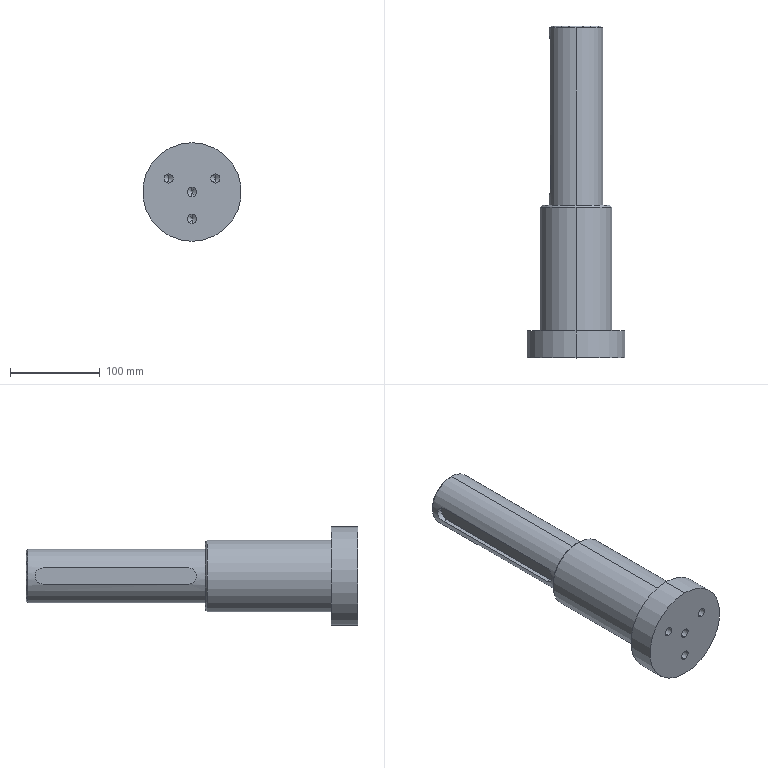Part | SolidWorks | features HoleWzd 2, ICE 2, Chamfer 1, Fillet 1, Revolution 1 | 1 solid | 41 faces | box 110 x 370 x 110 mm | volume 1516861 mm3 | cylinder 20 | cone 14 | plane 7 | commonest cylinder face diameters 10.2 x8 18 x4 15.5 x2 60 x2 80 x2 110 x2
STEP:
#1=CARTESIAN_POINT('',(0.,32.75,-24.9));
#2=VERTEX_POINT('',#1);
#3=CARTESIAN_POINT('',(0.,32.75,-35.1));
#4=VERTEX_POINT('',#3);
#5=CARTESIAN_POINT('',(0.,32.75,-30.));
#6=DIRECTION('',(0.,-1.,0.));
#7=DIRECTION('',(0.,0.,-1.));
#8=AXIS2_PLACEMENT_3D('',#5,#6,#7);
#9=CIRCLE('',#8,5.1);
#10=EDGE_CURVE('',#2,#4,#9,.T.);
#11=ORIENTED_EDGE('',*,*,#10,.F.);
#12=CARTESIAN_POINT('',(0.,0.,-24.9));
#13=VERTEX_POINT('',#12);
#14=CARTESIAN_POINT('',(0.,0.,-24.9));
#15=DIRECTION('',(0.,-1.,0.));
#16=VECTOR('',#15,1000.);
#17=LINE('',#14,#16);
#18=EDGE_CURVE('',#2,#13,#17,.T.);
#19=ORIENTED_EDGE('',*,*,#18,.T.);
#20=CARTESIAN_POINT('',(0.,0.,-35.1));
#21=VERTEX_POINT('',#20);
#22=CARTESIAN_POINT('',(0.,0.,-30.));
#23=DIRECTION('',(0.,-1.,0.));
#24=DIRECTION('',(0.,0.,-1.));
#25=AXIS2_PLACEMENT_3D('',#22,#23,#24);
#26=CIRCLE('',#25,5.1);
#27=EDGE_CURVE('',#13,#21,#26,.T.);
#28=ORIENTED_EDGE('',*,*,#27,.T.);
#29=CARTESIAN_POINT('',(0.,0.,-35.1));
#30=DIRECTION('',(0.,-1.,0.));
#31=VECTOR('',#30,1000.);
#32=LINE('',#29,#31);
#33=EDGE_CURVE('',#4,#21,#32,.T.);
#34=ORIENTED_EDGE('',*,*,#33,.F.);
#35=EDGE_LOOP('',(#11,#19,#28,#34));
#36=FACE_OUTER_BOUND('',#35,.T.);
#37=CARTESIAN_POINT('',(0.,0.,-30.));
#38=DIRECTION('',(0.,-1.,0.));
#39=DIRECTION('',(0.,0.,-1.));
#40=AXIS2_PLACEMENT_3D('',#37,#38,#39);
#41=CYLINDRICAL_SURFACE('',#40,5.1);
#42=ADVANCED_FACE('',(#36),#41,.F.);
#43=CARTESIAN_POINT('',(-25.981,32.75,20.1));
#44=VERTEX_POINT('',#43);
#45=CARTESIAN_POINT('',(-25.981,32.75,9.9));
#46=VERTEX_POINT('',#45);
#47=CARTESIAN_POINT('',(-25.981,32.75,15.));
#48=DIRECTION('',(0.,-1.,0.));
#49=DIRECTION('',(0.,0.,-1.));
#50=AXIS2_PLACEMENT_3D('',#47,#48,#49);
#51=CIRCLE('',#50,5.1);
#52=EDGE_CURVE('',#44,#46,#51,.T.);
#53=ORIENTED_EDGE('',*,*,#52,.F.);
#54=CARTESIAN_POINT('',(-25.981,0.,20.1));
#55=VERTEX_POINT('',#54);
#56=CARTESIAN_POINT('',(-25.981,0.,20.1));
#57=DIRECTION('',(0.,-1.,0.));
#58=VECTOR('',#57,1000.);
#59=LINE('',#56,#58);
#60=EDGE_CURVE('',#44,#55,#59,.T.);
#61=ORIENTED_EDGE('',*,*,#60,.T.);
#62=CARTESIAN_POINT('',(-25.981,0.,9.9));
#63=VERTEX_POINT('',#62);
#64=CARTESIAN_POINT('',(-25.981,0.,15.));
#65=DIRECTION('',(0.,-1.,0.));
#66=DIRECTION('',(0.,0.,-1.));
#67=AXIS2_PLACEMENT_3D('',#64,#65,#66);
#68=CIRCLE('',#67,5.1);
#69=EDGE_CURVE('',#55,#63,#68,.T.);
#70=ORIENTED_EDGE('',*,*,#69,.T.);
#71=CARTESIAN_POINT('',(-25.981,0.,9.9));
#72=DIRECTION('',(0.,-1.,0.));
#73=VECTOR('',#72,1000.);
#74=LINE('',#71,#73);
#75=EDGE_CURVE('',#46,#63,#74,.T.);
#76=ORIENTED_EDGE('',*,*,#75,.F.);
#77=EDGE_LOOP('',(#53,#61,#70,#76));
#78=FACE_OUTER_BOUND('',#77,.T.);
#79=CARTESIAN_POINT('',(-25.981,0.,15.));
#80=DIRECTION('',(0.,-1.,0.));
#81=DIRECTION('',(0.,0.,-1.));
#82=AXIS2_PLACEMENT_3D('',#79,#80,#81);
#83=CYLINDRICAL_SURFACE('',#82,5.1);
#84=ADVANCED_FACE('',(#78),#83,.F.);
#85=CARTESIAN_POINT('',(25.981,32.75,20.1));
#86=VERTEX_POINT('',#85);
#87=CARTESIAN_POINT('',(25.981,32.75,9.9));
#88=VERTEX_POINT('',#87);
#89=CARTESIAN_POINT('',(25.981,32.75,15.));
#90=DIRECTION('',(0.,-1.,0.));
#91=DIRECTION('',(0.,0.,-1.));
#92=AXIS2_PLACEMENT_3D('',#89,#90,#91);
#93=CIRCLE('',#92,5.1);
#94=EDGE_CURVE('',#86,#88,#93,.T.);
#95=ORIENTED_EDGE('',*,*,#94,.F.);
#96=CARTESIAN_POINT('',(25.981,0.,20.1));
#97=VERTEX_POINT('',#96);
#98=CARTESIAN_POINT('',(25.981,0.,20.1));
#99=DIRECTION('',(0.,-1.,0.));
#100=VECTOR('',#99,1000.);
#101=LINE('',#98,#100);
#102=EDGE_CURVE('',#86,#97,#101,.T.);
#103=ORIENTED_EDGE('',*,*,#102,.T.);
#104=CARTESIAN_POINT('',(25.981,0.,9.9));
#105=VERTEX_POINT('',#104);
#106=CARTESIAN_POINT('',(25.981,0.,15.));
#107=DIRECTION('',(0.,-1.,0.));
#108=DIRECTION('',(0.,0.,-1.));
#109=AXIS2_PLACEMENT_3D('',#106,#107,#108);
#110=CIRCLE('',#109,5.1);
#111=EDGE_CURVE('',#97,#105,#110,.T.);
#112=ORIENTED_EDGE('',*,*,#111,.T.);
#113=CARTESIAN_POINT('',(25.981,0.,9.9));
#114=DIRECTION('',(0.,-1.,0.));
#115=VECTOR('',#114,1000.);
#116=LINE('',#113,#115);
#117=EDGE_CURVE('',#88,#105,#116,.T.);
#118=ORIENTED_EDGE('',*,*,#117,.F.);
#119=EDGE_LOOP('',(#95,#103,#112,#118));
#120=FACE_OUTER_BOUND('',#119,.T.);
#121=CARTESIAN_POINT('',(25.981,0.,15.));
#122=DIRECTION('',(0.,-1.,0.));
#123=DIRECTION('',(0.,0.,-1.));
#124=AXIS2_PLACEMENT_3D('',#121,#122,#123);
#125=CYLINDRICAL_SURFACE('',#124,5.1);
#126=ADVANCED_FACE('',(#120),#125,.F.);
#127=CARTESIAN_POINT('',(0.,32.75,5.1));
#128=VERTEX_POINT('',#127);
#129=CARTESIAN_POINT('',(0.,32.75,-5.1));
#130=VERTEX_POINT('',#129);
#131=CARTESIAN_POINT('',(0.,32.75,0.));
#132=DIRECTION('',(0.,-1.,0.));
#133=DIRECTION('',(0.,0.,-1.));
#134=AXIS2_PLACEMENT_3D('',#131,#132,#133);
#135=CIRCLE('',#134,5.1);
#136=EDGE_CURVE('',#128,#130,#135,.T.);
#137=ORIENTED_EDGE('',*,*,#136,.F.);
#138=CARTESIAN_POINT('',(0.,0.,5.1));
#139=VERTEX_POINT('',#138);
#140=CARTESIAN_POINT('',(0.,0.,5.1));
#141=DIRECTION('',(0.,-1.,0.));
#142=VECTOR('',#141,1000.);
#143=LINE('',#140,#142);
#144=EDGE_CURVE('',#128,#139,#143,.T.);
#145=ORIENTED_EDGE('',*,*,#144,.T.);
#146=CARTESIAN_POINT('',(0.,0.,-5.1));
#147=VERTEX_POINT('',#146);
#148=CARTESIAN_POINT('',(0.,0.,0.));
#149=DIRECTION('',(0.,-1.,0.));
#150=DIRECTION('',(0.,0.,-1.));
#151=AXIS2_PLACEMENT_3D('',#148,#149,#150);
#152=CIRCLE('',#151,5.1);
#153=EDGE_CURVE('',#139,#147,#152,.T.);
#154=ORIENTED_EDGE('',*,*,#153,.T.);
#155=CARTESIAN_POINT('',(0.,0.,-5.1));
#156=DIRECTION('',(0.,-1.,0.));
#157=VECTOR('',#156,1000.);
#158=LINE('',#155,#157);
#159=EDGE_CURVE('',#130,#147,#158,.T.);
#160=ORIENTED_EDGE('',*,*,#159,.F.);
#161=EDGE_LOOP('',(#137,#145,#154,#160));
#162=FACE_OUTER_BOUND('',#161,.T.);
#163=CARTESIAN_POINT('',(0.,0.,0.));
#164=DIRECTION('',(0.,-1.,0.));
#165=DIRECTION('',(0.,0.,-1.));
#166=AXIS2_PLACEMENT_3D('',#163,#164,#165);
#167=CYLINDRICAL_SURFACE('',#166,5.1);
#168=ADVANCED_FACE('',(#162),#167,.F.);
#169=CARTESIAN_POINT('',(0.,35.814,-30.));
#170=VERTEX_POINT('',#169);
#171=CARTESIAN_POINT('',(0.,32.75,-35.1));
#172=DIRECTION('',(0.,-0.515,-0.8572));
#173=VECTOR('',#172,1000.);
#174=LINE('',#171,#173);
#175=EDGE_CURVE('',#170,#4,#174,.T.);
#176=ORIENTED_EDGE('',*,*,#175,.F.);
#177=CARTESIAN_POINT('',(0.,32.75,-24.9));
#178=DIRECTION('',(0.,-0.515,0.8572));
#179=VECTOR('',#178,1000.);
#180=LINE('',#177,#179);
#181=EDGE_CURVE('',#170,#2,#180,.T.);
#182=ORIENTED_EDGE('',*,*,#181,.T.);
#183=ORIENTED_EDGE('',*,*,#10,.T.);
#184=EDGE_LOOP('',(#176,#182,#183));
#185=FACE_OUTER_BOUND('',#184,.T.);
#186=CARTESIAN_POINT('',(0.,32.75,-30.));
#187=DIRECTION('',(0.,-1.,0.));
#188=DIRECTION('',(0.,0.,-1.));
#189=AXIS2_PLACEMENT_3D('',#186,#187,#188);
#190=CONICAL_SURFACE('',#189,5.1,1.03);
#191=ADVANCED_FACE('',(#185),#190,.F.);
#192=CARTESIAN_POINT('',(-25.981,35.814,15.));
#193=VERTEX_POINT('',#192);
#194=CARTESIAN_POINT('',(-25.981,32.75,9.9));
#195=DIRECTION('',(0.,-0.515,-0.8572));
#196=VECTOR('',#195,1000.);
#197=LINE('',#194,#196);
#198=EDGE_CURVE('',#193,#46,#197,.T.);
#199=ORIENTED_EDGE('',*,*,#198,.F.);
#200=CARTESIAN_POINT('',(-25.981,32.75,20.1));
#201=DIRECTION('',(0.,-0.515,0.8572));
#202=VECTOR('',#201,1000.);
#203=LINE('',#200,#202);
#204=EDGE_CURVE('',#193,#44,#203,.T.);
#205=ORIENTED_EDGE('',*,*,#204,.T.);
#206=ORIENTED_EDGE('',*,*,#52,.T.);
#207=EDGE_LOOP('',(#199,#205,#206));
#208=FACE_OUTER_BOUND('',#207,.T.);
#209=CARTESIAN_POINT('',(-25.981,32.75,15.));
#210=DIRECTION('',(0.,-1.,0.));
#211=DIRECTION('',(0.,0.,-1.));
#212=AXIS2_PLACEMENT_3D('',#209,#210,#211);
#213=CONICAL_SURFACE('',#212,5.1,1.03);
#214=ADVANCED_FACE('',(#208),#213,.F.);
#215=CARTESIAN_POINT('',(25.981,35.814,15.));
#216=VERTEX_POINT('',#215);
#217=CARTESIAN_POINT('',(25.981,32.75,9.9));
#218=DIRECTION('',(0.,-0.515,-0.8572));
#219=VECTOR('',#218,1000.);
#220=LINE('',#217,#219);
#221=EDGE_CURVE('',#216,#88,#220,.T.);
#222=ORIENTED_EDGE('',*,*,#221,.F.);
#223=CARTESIAN_POINT('',(25.981,32.75,20.1));
#224=DIRECTION('',(0.,-0.515,0.8572));
#225=VECTOR('',#224,1000.);
#226=LINE('',#223,#225);
#227=EDGE_CURVE('',#216,#86,#226,.T.);
#228=ORIENTED_EDGE('',*,*,#227,.T.);
#229=ORIENTED_EDGE('',*,*,#94,.T.);
#230=EDGE_LOOP('',(#222,#228,#229));
#231=FACE_OUTER_BOUND('',#230,.T.);
#232=CARTESIAN_POINT('',(25.981,32.75,15.));
#233=DIRECTION('',(0.,-1.,0.));
#234=DIRECTION('',(0.,0.,-1.));
#235=AXIS2_PLACEMENT_3D('',#232,#233,#234);
#236=CONICAL_SURFACE('',#235,5.1,1.03);
#237=ADVANCED_FACE('',(#231),#236,.F.);
#238=CARTESIAN_POINT('',(0.,35.814,0.));
#239=VERTEX_POINT('',#238);
#240=CARTESIAN_POINT('',(0.,32.75,-5.1));
#241=DIRECTION('',(0.,-0.515,-0.8572));
#242=VECTOR('',#241,1000.);
#243=LINE('',#240,#242);
#244=EDGE_CURVE('',#239,#130,#243,.T.);
#245=ORIENTED_EDGE('',*,*,#244,.F.);
#246=CARTESIAN_POINT('',(0.,32.75,5.1));
#247=DIRECTION('',(0.,-0.515,0.8572));
#248=VECTOR('',#247,1000.);
#249=LINE('',#246,#248);
#250=EDGE_CURVE('',#239,#128,#249,.T.);
#251=ORIENTED_EDGE('',*,*,#250,.T.);
#252=ORIENTED_EDGE('',*,*,#136,.T.);
#253=EDGE_LOOP('',(#245,#251,#252));
#254=FACE_OUTER_BOUND('',#253,.T.);
#255=CARTESIAN_POINT('',(0.,32.75,0.));
#256=DIRECTION('',(0.,-1.,0.));
#257=DIRECTION('',(0.,0.,-1.));
#258=AXIS2_PLACEMENT_3D('',#255,#256,#257);
#259=CONICAL_SURFACE('',#258,5.1,1.03);
#260=ADVANCED_FACE('',(#254),#259,.F.);
#261=CARTESIAN_POINT('',(0.,30.,-55.));
#262=VERTEX_POINT('',#261);
#263=CARTESIAN_POINT('',(0.,30.,55.));
#264=VERTEX_POINT('',#263);
#265=CARTESIAN_POINT('',(0.,30.,0.));
#266=DIRECTION('',(0.,-1.,0.));
#267=DIRECTION('',(0.,0.,-1.));
#268=AXIS2_PLACEMENT_3D('',#265,#266,#267);
#269=CIRCLE('',#268,55.);
#270=EDGE_CURVE('',#262,#264,#269,.T.);
#271=ORIENTED_EDGE('',*,*,#270,.T.);
#272=CARTESIAN_POINT('',(0.,0.,55.));
#273=VERTEX_POINT('',#272);
#274=CARTESIAN_POINT('',(0.,30.,55.));
#275=DIRECTION('',(0.,-1.,0.));
#276=VECTOR('',#275,1000.);
#277=LINE('',#274,#276);
#278=EDGE_CURVE('',#264,#273,#277,.T.);
#279=ORIENTED_EDGE('',*,*,#278,.T.);
#280=CARTESIAN_POINT('',(0.,0.,-55.));
#281=VERTEX_POINT('',#280);
#282=CARTESIAN_POINT('',(0.,0.,0.));
#283=DIRECTION('',(0.,-1.,0.));
#284=DIRECTION('',(0.,0.,-1.));
#285=AXIS2_PLACEMENT_3D('',#282,#283,#284);
#286=CIRCLE('',#285,55.);
#287=EDGE_CURVE('',#281,#273,#286,.T.);
#288=ORIENTED_EDGE('',*,*,#287,.F.);
#289=CARTESIAN_POINT('',(0.,30.,-55.));
#290=DIRECTION('',(0.,-1.,0.));
#291=VECTOR('',#290,1000.);
#292=LINE('',#289,#291);
#293=EDGE_CURVE('',#262,#281,#292,.T.);
#294=ORIENTED_EDGE('',*,*,#293,.F.);
#295=EDGE_LOOP('',(#271,#279,#288,#294));
#296=FACE_OUTER_BOUND('',#295,.T.);
#297=CARTESIAN_POINT('',(0.,30.,0.));
#298=DIRECTION('',(0.,-1.,0.));
#299=DIRECTION('',(0.,0.,-1.));
#300=AXIS2_PLACEMENT_3D('',#297,#298,#299);
#301=CYLINDRICAL_SURFACE('',#300,55.);
#302=ADVANCED_FACE('',(#296),#301,.T.);
#303=CARTESIAN_POINT('',(0.,370.,28.));
#304=VERTEX_POINT('',#303);
#305=CARTESIAN_POINT('',(0.,370.,-28.));
#306=VERTEX_POINT('',#305);
#307=CARTESIAN_POINT('',(0.,370.,0.));
#308=DIRECTION('',(0.,1.,0.));
#309=DIRECTION('',(0.,0.,1.));
#310=AXIS2_PLACEMENT_3D('',#307,#308,#309);
#311=CIRCLE('',#310,28.);
#312=EDGE_CURVE('',#304,#306,#311,.T.);
#313=ORIENTED_EDGE('',*,*,#312,.F.);
#314=CARTESIAN_POINT('',(0.,368.,30.));
#315=VERTEX_POINT('',#314);
#316=CARTESIAN_POINT('',(0.,368.,30.));
#317=DIRECTION('',(0.,-0.7071,0.7071));
#318=VECTOR('',#317,1000.);
#319=LINE('',#316,#318);
#320=EDGE_CURVE('',#304,#315,#319,.T.);
#321=ORIENTED_EDGE('',*,*,#320,.T.);
#322=CARTESIAN_POINT('',(0.,368.,-30.));
#323=VERTEX_POINT('',#322);
#324=CARTESIAN_POINT('',(0.,368.,0.));
#325=DIRECTION('',(0.,-1.,0.));
#326=DIRECTION('',(0.,0.,1.));
#327=AXIS2_PLACEMENT_3D('',#324,#325,#326);
#328=CIRCLE('',#327,30.);
#329=EDGE_CURVE('',#323,#315,#328,.T.);
#330=ORIENTED_EDGE('',*,*,#329,.F.);
#331=CARTESIAN_POINT('',(0.,368.,-30.));
#332=DIRECTION('',(0.,-0.7071,-0.7071));
#333=VECTOR('',#332,1000.);
#334=LINE('',#331,#333);
#335=EDGE_CURVE('',#306,#323,#334,.T.);
#336=ORIENTED_EDGE('',*,*,#335,.F.);
#337=EDGE_LOOP('',(#313,#321,#330,#336));
#338=FACE_OUTER_BOUND('',#337,.T.);
#339=CARTESIAN_POINT('',(0.,368.,0.));
#340=DIRECTION('',(0.,-1.,0.));
#341=DIRECTION('',(0.,0.,-1.));
#342=AXIS2_PLACEMENT_3D('',#339,#340,#341);
#343=CONICAL_SURFACE('',#342,30.,0.7854);
#344=ADVANCED_FACE('',(#338),#343,.T.);
#345=CARTESIAN_POINT('',(0.,170.,38.));
#346=VERTEX_POINT('',#345);
#347=CARTESIAN_POINT('',(0.,170.,-38.));
#348=VERTEX_POINT('',#347);
#349=CARTESIAN_POINT('',(0.,170.,0.));
#350=DIRECTION('',(0.,1.,0.));
#351=DIRECTION('',(0.,0.,1.));
#352=AXIS2_PLACEMENT_3D('',#349,#350,#351);
#353=CIRCLE('',#352,38.);
#354=EDGE_CURVE('',#346,#348,#353,.T.);
#355=ORIENTED_EDGE('',*,*,#354,.F.);
#356=CARTESIAN_POINT('',(0.,168.,40.));
#357=VERTEX_POINT('',#356);
#358=CARTESIAN_POINT('',(0.,168.,40.));
#359=DIRECTION('',(0.,-0.7071,0.7071));
#360=VECTOR('',#359,1000.);
#361=LINE('',#358,#360);
#362=EDGE_CURVE('',#346,#357,#361,.T.);
#363=ORIENTED_EDGE('',*,*,#362,.T.);
#364=CARTESIAN_POINT('',(0.,168.,-40.));
#365=VERTEX_POINT('',#364);
#366=CARTESIAN_POINT('',(0.,168.,0.));
#367=DIRECTION('',(0.,-1.,0.));
#368=DIRECTION('',(0.,0.,1.));
#369=AXIS2_PLACEMENT_3D('',#366,#367,#368);
#370=CIRCLE('',#369,40.);
#371=EDGE_CURVE('',#365,#357,#370,.T.);
#372=ORIENTED_EDGE('',*,*,#371,.F.);
#373=CARTESIAN_POINT('',(0.,168.,-40.));
#374=DIRECTION('',(0.,-0.7071,-0.7071));
#375=VECTOR('',#374,1000.);
#376=LINE('',#373,#375);
#377=EDGE_CURVE('',#348,#365,#376,.T.);
#378=ORIENTED_EDGE('',*,*,#377,.F.);
#379=EDGE_LOOP('',(#355,#363,#372,#378));
#380=FACE_OUTER_BOUND('',#379,.T.);
#381=CARTESIAN_POINT('',(0.,168.,0.));
#382=DIRECTION('',(0.,-1.,0.));
#383=DIRECTION('',(0.,0.,-1.));
#384=AXIS2_PLACEMENT_3D('',#381,#382,#383);
#385=CONICAL_SURFACE('',#384,40.,0.7854);
#386=ADVANCED_FACE('',(#380),#385,.T.);
#387=CARTESIAN_POINT('',(0.,329.5,-7.75));
#388=VERTEX_POINT('',#387);
#389=CARTESIAN_POINT('',(0.,329.5,7.75));
#390=VERTEX_POINT('',#389);
#391=CARTESIAN_POINT('',(0.,329.5,0.));
#392=DIRECTION('',(0.,1.,0.));
#393=DIRECTION('',(0.,0.,1.));
#394=AXIS2_PLACEMENT_3D('',#391,#392,#393);
#395=CIRCLE('',#394,7.75);
#396=EDGE_CURVE('',#388,#390,#395,.T.);
#397=ORIENTED_EDGE('',*,*,#396,.F.);
#398=CARTESIAN_POINT('',(0.,370.,-7.75));
#399=VERTEX_POINT('',#398);
#400=CARTESIAN_POINT('',(0.,370.,-7.75));
#401=DIRECTION('',(0.,1.,0.));
#402=VECTOR('',#401,1000.);
#403=LINE('',#400,#402);
#404=EDGE_CURVE('',#388,#399,#403,.T.);
#405=ORIENTED_EDGE('',*,*,#404,.T.);
#406=CARTESIAN_POINT('',(0.,370.,7.75));
#407=VERTEX_POINT('',#406);
#408=CARTESIAN_POINT('',(0.,370.,0.));
#409=DIRECTION('',(0.,1.,0.));
#410=DIRECTION('',(0.,0.,1.));
#411=AXIS2_PLACEMENT_3D('',#408,#409,#410);
#412=CIRCLE('',#411,7.75);
#413=EDGE_CURVE('',#399,#407,#412,.T.);
#414=ORIENTED_EDGE('',*,*,#413,.T.);
#415=CARTESIAN_POINT('',(0.,370.,7.75));
#416=DIRECTION('',(0.,1.,0.));
#417=VECTOR('',#416,1000.);
#418=LINE('',#415,#417);
#419=EDGE_CURVE('',#390,#407,#418,.T.);
#420=ORIENTED_EDGE('',*,*,#419,.F.);
#421=EDGE_LOOP('',(#397,#405,#414,#420));
#422=FACE_OUTER_BOUND('',#421,.T.);
#423=CARTESIAN_POINT('',(0.,370.,0.));
#424=DIRECTION('',(0.,1.,0.));
#425=DIRECTION('',(0.,0.,1.));
#426=AXIS2_PLACEMENT_3D('',#423,#424,#425);
#427=CYLINDRICAL_SURFACE('',#426,7.75);
#428=ADVANCED_FACE('',(#422),#427,.F.);
#429=CARTESIAN_POINT('',(0.,324.843,0.));
#430=VERTEX_POINT('',#429);
#431=CARTESIAN_POINT('',(0.,329.5,7.75));
#432=DIRECTION('',(0.,0.515,0.8572));
#433=VECTOR('',#432,1000.);
#434=LINE('',#431,#433);
#435=EDGE_CURVE('',#430,#390,#434,.T.);
#436=ORIENTED_EDGE('',*,*,#435,.F.);
#437=CARTESIAN_POINT('',(0.,329.5,-7.75));
#438=DIRECTION('',(0.,0.515,-0.8572));
#439=VECTOR('',#438,1000.);
#440=LINE('',#437,#439);
#441=EDGE_CURVE('',#430,#388,#440,.T.);
#442=ORIENTED_EDGE('',*,*,#441,.T.);
#443=ORIENTED_EDGE('',*,*,#396,.T.);
#444=EDGE_LOOP('',(#436,#442,#443));
#445=FACE_OUTER_BOUND('',#444,.T.);
#446=CARTESIAN_POINT('',(0.,329.5,0.));
#447=DIRECTION('',(0.,1.,0.));
#448=DIRECTION('',(0.,0.,1.));
#449=AXIS2_PLACEMENT_3D('',#446,#447,#448);
#450=CONICAL_SURFACE('',#449,7.75,1.03);
#451=ADVANCED_FACE('',(#445),#450,.F.);
#452=ORIENTED_EDGE('',*,*,#329,.T.);
#453=CARTESIAN_POINT('',(0.,170.,30.));
#454=VERTEX_POINT('',#453);
#455=CARTESIAN_POINT('',(0.,0.,30.));
#456=DIRECTION('',(0.,-1.,0.));
#457=VECTOR('',#456,1000.);
#458=LINE('',#455,#457);
#459=EDGE_CURVE('',#315,#454,#458,.T.);
#460=ORIENTED_EDGE('',*,*,#459,.T.);
#461=CARTESIAN_POINT('',(0.,170.,-30.));
#462=VERTEX_POINT('',#461);
#463=CARTESIAN_POINT('',(0.,170.,0.));
#464=DIRECTION('',(0.,-1.,0.));
#465=DIRECTION('',(0.,0.,-1.));
#466=AXIS2_PLACEMENT_3D('',#463,#464,#465);
#467=CIRCLE('',#466,30.);
#468=EDGE_CURVE('',#462,#454,#467,.T.);
#469=ORIENTED_EDGE('',*,*,#468,.F.);
#470=CARTESIAN_POINT('',(0.,0.,-30.));
#471=DIRECTION('',(0.,-1.,0.));
#472=VECTOR('',#471,1000.);
#473=LINE('',#470,#472);
#474=EDGE_CURVE('',#323,#462,#473,.T.);
#475=ORIENTED_EDGE('',*,*,#474,.F.);
#476=EDGE_LOOP('',(#452,#460,#469,#475));
#477=FACE_OUTER_BOUND('',#476,.T.);
#478=CARTESIAN_POINT('',(0.,0.,0.));
#479=DIRECTION('',(0.,-1.,0.));
#480=DIRECTION('',(0.,0.,-1.));
#481=AXIS2_PLACEMENT_3D('',#478,#479,#480);
#482=CYLINDRICAL_SURFACE('',#481,30.);
#483=ADVANCED_FACE('',(#477),#482,.T.);
#484=ORIENTED_EDGE('',*,*,#371,.T.);
#485=CARTESIAN_POINT('',(0.,30.,40.));
#486=VERTEX_POINT('',#485);
#487=CARTESIAN_POINT('',(0.,0.,40.));
#488=DIRECTION('',(0.,-1.,0.));
#489=VECTOR('',#488,1000.);
#490=LINE('',#487,#489);
#491=EDGE_CURVE('',#357,#486,#490,.T.);
#492=ORIENTED_EDGE('',*,*,#491,.T.);
#493=CARTESIAN_POINT('',(0.,30.,-40.));
#494=VERTEX_POINT('',#493);
#495=CARTESIAN_POINT('',(0.,30.,0.));
#496=DIRECTION('',(0.,-1.,0.));
#497=DIRECTION('',(0.,0.,-1.));
#498=AXIS2_PLACEMENT_3D('',#495,#496,#497);
#499=CIRCLE('',#498,40.);
#500=EDGE_CURVE('',#494,#486,#499,.T.);
#501=ORIENTED_EDGE('',*,*,#500,.F.);
#502=CARTESIAN_POINT('',(0.,0.,-40.));
#503=DIRECTION('',(0.,-1.,0.));
#504=VECTOR('',#503,1000.);
#505=LINE('',#502,#504);
#506=EDGE_CURVE('',#365,#494,#505,.T.);
#507=ORIENTED_EDGE('',*,*,#506,.F.);
#508=EDGE_LOOP('',(#484,#492,#501,#507));
#509=FACE_OUTER_BOUND('',#508,.T.);
#510=CARTESIAN_POINT('',(0.,0.,0.));
#511=DIRECTION('',(0.,-1.,0.));
#512=DIRECTION('',(0.,0.,-1.));
#513=AXIS2_PLACEMENT_3D('',#510,#511,#512);
#514=CYLINDRICAL_SURFACE('',#513,40.);
#515=ADVANCED_FACE('',(#509),#514,.T.);
#516=ORIENTED_EDGE('',*,*,#491,.F.);
#517=CARTESIAN_POINT('',(0.,168.,0.));
#518=DIRECTION('',(0.,-1.,0.));
#519=DIRECTION('',(0.,0.,1.));
#520=AXIS2_PLACEMENT_3D('',#517,#518,#519);
#521=CIRCLE('',#520,40.);
#522=EDGE_CURVE('',#357,#365,#521,.T.);
#523=ORIENTED_EDGE('',*,*,#522,.T.);
#524=ORIENTED_EDGE('',*,*,#506,.T.);
#525=CARTESIAN_POINT('',(0.,30.,0.));
#526=DIRECTION('',(0.,-1.,0.));
#527=DIRECTION('',(0.,0.,-1.));
#528=AXIS2_PLACEMENT_3D('',#525,#526,#527);
#529=CIRCLE('',#528,40.);
#530=EDGE_CURVE('',#486,#494,#529,.T.);
#531=ORIENTED_EDGE('',*,*,#530,.F.);
#532=EDGE_LOOP('',(#516,#523,#524,#531));
#533=FACE_OUTER_BOUND('',#532,.T.);
#534=CARTESIAN_POINT('',(0.,0.,0.));
#535=DIRECTION('',(0.,-1.,0.));
#536=DIRECTION('',(0.,0.,-1.));
#537=AXIS2_PLACEMENT_3D('',#534,#535,#536);
#538=CYLINDRICAL_SURFACE('',#537,40.);
#539=ADVANCED_FACE('',(#533),#538,.T.);
#540=CARTESIAN_POINT('',(0.,370.,0.));
#541=DIRECTION('',(0.,1.,0.));
#542=DIRECTION('',(0.,0.,1.));
#543=AXIS2_PLACEMENT_3D('',#540,#541,#542);
#544=CIRCLE('',#543,28.);
#545=EDGE_CURVE('',#306,#304,#544,.T.);
#546=ORIENTED_EDGE('',*,*,#545,.T.);
#547=ORIENTED_EDGE('',*,*,#312,.T.);
#548=EDGE_LOOP('',(#546,#547));
#549=FACE_OUTER_BOUND('',#548,.T.);
#550=CARTESIAN_POINT('',(0.,370.,0.));
#551=DIRECTION('',(0.,1.,0.));
#552=DIRECTION('',(0.,0.,1.));
#553=AXIS2_PLACEMENT_3D('',#550,#551,#552);
#554=CIRCLE('',#553,7.75);
#555=EDGE_CURVE('',#407,#399,#554,.T.);
#556=ORIENTED_EDGE('',*,*,#555,.F.);
#557=ORIENTED_EDGE('',*,*,#413,.F.);
#558=EDGE_LOOP('',(#556,#557));
#559=FACE_BOUND('',#558,.T.);
#560=CARTESIAN_POINT('',(0.,370.,0.));
#561=DIRECTION('',(0.,1.,0.));
#562=DIRECTION('',(0.,0.,1.));
#563=AXIS2_PLACEMENT_3D('',#560,#561,#562);
#564=PLANE('',#563);
#565=ADVANCED_FACE('',(#549,#559),#564,.T.);
#566=ORIENTED_EDGE('',*,*,#459,.F.);
#567=CARTESIAN_POINT('',(0.,368.,0.));
#568=DIRECTION('',(0.,-1.,0.));
#569=DIRECTION('',(0.,0.,1.));
#570=AXIS2_PLACEMENT_3D('',#567,#568,#569);
#571=CIRCLE('',#570,30.);
#572=EDGE_CURVE('',#315,#323,#571,.T.);
#573=ORIENTED_EDGE('',*,*,#572,.T.);
#574=ORIENTED_EDGE('',*,*,#474,.T.);
#575=CARTESIAN_POINT('',(0.,170.,0.));
#576=DIRECTION('',(0.,-1.,0.));
#577=DIRECTION('',(0.,0.,-1.));
#578=AXIS2_PLACEMENT_3D('',#575,#576,#577);
#579=CIRCLE('',#578,30.);
#580=EDGE_CURVE('',#454,#462,#579,.T.);
#581=ORIENTED_EDGE('',*,*,#580,.F.);
#582=EDGE_LOOP('',(#566,#573,#574,#581));
#583=FACE_OUTER_BOUND('',#582,.T.);
#584=CARTESIAN_POINT('',(-28.618,189.,9.));
#585=VERTEX_POINT('',#584);
#586=CARTESIAN_POINT('',(-28.618,351.,9.));
#587=VERTEX_POINT('',#586);
#588=CARTESIAN_POINT('',(-28.618,0.,9.));
#589=DIRECTION('',(0.,1.,0.));
#590=VECTOR('',#589,1000.);
#591=LINE('',#588,#590);
#592=EDGE_CURVE('',#585,#587,#591,.T.);
#593=ORIENTED_EDGE('',*,*,#592,.F.);
#594=CARTESIAN_POINT('',(-30.,180.,0.));
#595=VERTEX_POINT('',#594);
#596=CARTESIAN_POINT('',(-28.618,189.,9.));
#597=CARTESIAN_POINT('',(-28.618,188.402,9.));
#598=CARTESIAN_POINT('',(-28.637,187.815,8.941));
#599=CARTESIAN_POINT('',(-28.69,186.949,8.768));
#600=CARTESIAN_POINT('',(-28.712,186.663,8.696));
#601=CARTESIAN_POINT('',(-28.764,186.096,8.524));
#602=CARTESIAN_POINT('',(-28.794,185.816,8.423));
#603=CARTESIAN_POINT('',(-28.891,185.,8.084));
#604=CARTESIAN_POINT('',(-28.968,184.485,7.807));
#605=CARTESIAN_POINT('',(-29.094,183.753,7.318));
#606=CARTESIAN_POINT('',(-29.138,183.515,7.142));
#607=CARTESIAN_POINT('',(-29.227,183.061,6.768));
#608=CARTESIAN_POINT('',(-29.272,182.844,6.572));
#609=CARTESIAN_POINT('',(-29.406,182.226,5.954));
#610=CARTESIAN_POINT('',(-29.495,181.854,5.503));
#611=CARTESIAN_POINT('',(-29.661,181.196,4.522));
#612=CARTESIAN_POINT('',(-29.737,180.918,4.004));
#613=CARTESIAN_POINT('',(-29.831,180.58,3.193));
#614=CARTESIAN_POINT('',(-29.859,180.481,2.917));
#615=CARTESIAN_POINT('',(-29.909,180.308,2.352));
#616=CARTESIAN_POINT('',(-29.93,180.234,2.062));
#617=CARTESIAN_POINT('',(-29.982,180.059,1.188));
#618=CARTESIAN_POINT('',(-30.,180.,0.598));
#619=CARTESIAN_POINT('',(-30.,180.,0.));
#620=B_SPLINE_CURVE_WITH_KNOTS('',3,(#596,#597,#598,#599,#600,#601,#602,#603,#604,#605,#606,#607,#608,#609,#610,#611,#612,#613,#614,#615,#616,#617,#618,#619),.UNSPECIFIED.,.F.,.F.,(4,2,2,2,2,2,2,2,2,2,2,4),(0.,0.001768,0.002652,0.003535,0.005303,0.006187,0.007071,0.008838,0.01061,0.01149,0.01237,0.01414),.UNSPECIFIED.);
#621=EDGE_CURVE('',#585,#595,#620,.T.);
#622=ORIENTED_EDGE('',*,*,#621,.T.);
#623=CARTESIAN_POINT('',(-28.618,189.,-9.));
#624=VERTEX_POINT('',#623);
#625=CARTESIAN_POINT('',(-30.,180.,0.));
#626=CARTESIAN_POINT('',(-30.,180.,-0.598));
#627=CARTESIAN_POINT('',(-29.982,180.059,-1.185));
#628=CARTESIAN_POINT('',(-29.931,180.232,-2.051));
#629=CARTESIAN_POINT('',(-29.91,180.304,-2.337));
#630=CARTESIAN_POINT('',(-29.86,180.476,-2.904));
#631=CARTESIAN_POINT('',(-29.832,180.577,-3.185));
#632=CARTESIAN_POINT('',(-29.737,180.917,-4.001));
#633=CARTESIAN_POINT('',(-29.662,181.193,-4.516));
#634=CARTESIAN_POINT('',(-29.538,181.683,-5.248));
#635=CARTESIAN_POINT('',(-29.495,181.859,-5.486));
#636=CARTESIAN_POINT('',(-29.407,182.233,-5.94));
#637=CARTESIAN_POINT('',(-29.362,182.429,-6.157));
#638=CARTESIAN_POINT('',(-29.228,183.047,-6.775));
#639=CARTESIAN_POINT('',(-29.138,183.498,-7.147));
#640=CARTESIAN_POINT('',(-28.969,184.479,-7.805));
#641=CARTESIAN_POINT('',(-28.892,184.997,-8.082));
#642=CARTESIAN_POINT('',(-28.794,185.807,-8.42));
#643=CARTESIAN_POINT('',(-28.765,186.083,-8.519));
#644=CARTESIAN_POINT('',(-28.713,186.648,-8.692));
#645=CARTESIAN_POINT('',(-28.691,186.938,-8.766));
#646=CARTESIAN_POINT('',(-28.637,187.812,-8.941));
#647=CARTESIAN_POINT('',(-28.618,188.402,-9.));
#648=CARTESIAN_POINT('',(-28.618,189.,-9.));
#649=B_SPLINE_CURVE_WITH_KNOTS('',3,(#625,#626,#627,#628,#629,#630,#631,#632,#633,#634,#635,#636,#637,#638,#639,#640,#641,#642,#643,#644,#645,#646,#647,#648),.UNSPECIFIED.,.F.,.F.,(4,2,2,2,2,2,2,2,2,2,2,4),(0.,0.001768,0.002652,0.003535,0.005303,0.006187,0.007071,0.008839,0.01061,0.01149,0.01237,0.01414),.UNSPECIFIED.);
#650=EDGE_CURVE('',#595,#624,#649,.T.);
#651=ORIENTED_EDGE('',*,*,#650,.T.);
#652=CARTESIAN_POINT('',(-28.618,351.,-9.));
#653=VERTEX_POINT('',#652);
#654=CARTESIAN_POINT('',(-28.618,0.,-9.));
#655=DIRECTION('',(0.,-1.,0.));
#656=VECTOR('',#655,1000.);
#657=LINE('',#654,#656);
#658=EDGE_CURVE('',#653,#624,#657,.T.);
#659=ORIENTED_EDGE('',*,*,#658,.F.);
#660=CARTESIAN_POINT('',(-30.,360.,0.));
#661=VERTEX_POINT('',#660);
#662=CARTESIAN_POINT('',(-28.618,351.,-9.));
#663=CARTESIAN_POINT('',(-28.618,351.598,-9.));
#664=CARTESIAN_POINT('',(-28.637,352.185,-8.941));
#665=CARTESIAN_POINT('',(-28.69,353.051,-8.768));
#666=CARTESIAN_POINT('',(-28.712,353.337,-8.696));
#667=CARTESIAN_POINT('',(-28.764,353.904,-8.524));
#668=CARTESIAN_POINT('',(-28.794,354.184,-8.423));
#669=CARTESIAN_POINT('',(-28.891,355.,-8.084));
#670=CARTESIAN_POINT('',(-28.968,355.515,-7.807));
#671=CARTESIAN_POINT('',(-29.094,356.247,-7.318));
#672=CARTESIAN_POINT('',(-29.138,356.485,-7.142));
#673=CARTESIAN_POINT('',(-29.227,356.939,-6.768));
#674=CARTESIAN_POINT('',(-29.272,357.156,-6.572));
#675=CARTESIAN_POINT('',(-29.406,357.774,-5.954));
#676=CARTESIAN_POINT('',(-29.495,358.146,-5.503));
#677=CARTESIAN_POINT('',(-29.661,358.804,-4.522));
#678=CARTESIAN_POINT('',(-29.737,359.082,-4.004));
#679=CARTESIAN_POINT('',(-29.831,359.42,-3.193));
#680=CARTESIAN_POINT('',(-29.859,359.519,-2.917));
#681=CARTESIAN_POINT('',(-29.909,359.692,-2.352));
#682=CARTESIAN_POINT('',(-29.93,359.766,-2.062));
#683=CARTESIAN_POINT('',(-29.982,359.941,-1.188));
#684=CARTESIAN_POINT('',(-30.,360.,-0.598));
#685=CARTESIAN_POINT('',(-30.,360.,0.));
#686=B_SPLINE_CURVE_WITH_KNOTS('',3,(#662,#663,#664,#665,#666,#667,#668,#669,#670,#671,#672,#673,#674,#675,#676,#677,#678,#679,#680,#681,#682,#683,#684,#685),.UNSPECIFIED.,.F.,.F.,(4,2,2,2,2,2,2,2,2,2,2,4),(0.,0.001768,0.002652,0.003535,0.005303,0.006187,0.007071,0.008838,0.01061,0.01149,0.01237,0.01414),.UNSPECIFIED.);
#687=EDGE_CURVE('',#653,#661,#686,.T.);
#688=ORIENTED_EDGE('',*,*,#687,.T.);
#689=CARTESIAN_POINT('',(-30.,360.,0.));
#690=CARTESIAN_POINT('',(-30.,360.,0.598));
#691=CARTESIAN_POINT('',(-29.982,359.941,1.185));
#692=CARTESIAN_POINT('',(-29.931,359.768,2.051));
#693=CARTESIAN_POINT('',(-29.91,359.696,2.337));
#694=CARTESIAN_POINT('',(-29.86,359.524,2.904));
#695=CARTESIAN_POINT('',(-29.832,359.423,3.185));
#696=CARTESIAN_POINT('',(-29.737,359.083,4.001));
#697=CARTESIAN_POINT('',(-29.662,358.807,4.516));
#698=CARTESIAN_POINT('',(-29.538,358.317,5.248));
#699=CARTESIAN_POINT('',(-29.495,358.141,5.486));
#700=CARTESIAN_POINT('',(-29.407,357.767,5.94));
#701=CARTESIAN_POINT('',(-29.362,357.571,6.157));
#702=CARTESIAN_POINT('',(-29.228,356.953,6.775));
#703=CARTESIAN_POINT('',(-29.138,356.502,7.147));
#704=CARTESIAN_POINT('',(-28.969,355.521,7.805));
#705=CARTESIAN_POINT('',(-28.892,355.003,8.082));
#706=CARTESIAN_POINT('',(-28.794,354.193,8.42));
#707=CARTESIAN_POINT('',(-28.765,353.917,8.519));
#708=CARTESIAN_POINT('',(-28.713,353.352,8.692));
#709=CARTESIAN_POINT('',(-28.691,353.062,8.766));
#710=CARTESIAN_POINT('',(-28.637,352.188,8.941));
#711=CARTESIAN_POINT('',(-28.618,351.598,9.));
#712=CARTESIAN_POINT('',(-28.618,351.,9.));
#713=B_SPLINE_CURVE_WITH_KNOTS('',3,(#689,#690,#691,#692,#693,#694,#695,#696,#697,#698,#699,#700,#701,#702,#703,#704,#705,#706,#707,#708,#709,#710,#711,#712),.UNSPECIFIED.,.F.,.F.,(4,2,2,2,2,2,2,2,2,2,2,4),(0.,0.001768,0.002652,0.003535,0.005303,0.006187,0.007071,0.008839,0.01061,0.01149,0.01237,0.01414),.UNSPECIFIED.);
#714=EDGE_CURVE('',#661,#587,#713,.T.);
#715=ORIENTED_EDGE('',*,*,#714,.T.);
#716=EDGE_LOOP('',(#593,#622,#651,#659,#688,#715));
#717=FACE_BOUND('',#716,.T.);
#718=CARTESIAN_POINT('',(0.,0.,0.));
#719=DIRECTION('',(0.,-1.,0.));
#720=DIRECTION('',(0.,0.,-1.));
#721=AXIS2_PLACEMENT_3D('',#718,#719,#720);
#722=CYLINDRICAL_SURFACE('',#721,30.);
#723=ADVANCED_FACE('',(#583,#717),#722,.T.);
#724=CARTESIAN_POINT('',(0.,170.,0.));
#725=DIRECTION('',(0.,1.,0.));
#726=DIRECTION('',(0.,0.,1.));
#727=AXIS2_PLACEMENT_3D('',#724,#725,#726);
#728=CIRCLE('',#727,38.);
#729=EDGE_CURVE('',#348,#346,#728,.T.);
#730=ORIENTED_EDGE('',*,*,#729,.T.);
#731=ORIENTED_EDGE('',*,*,#354,.T.);
#732=EDGE_LOOP('',(#730,#731));
#733=FACE_OUTER_BOUND('',#732,.T.);
#734=ORIENTED_EDGE('',*,*,#468,.T.);
#735=ORIENTED_EDGE('',*,*,#580,.T.);
#736=EDGE_LOOP('',(#734,#735));
#737=FACE_BOUND('',#736,.T.);
#738=CARTESIAN_POINT('',(30.,170.,0.));
#739=DIRECTION('',(0.,1.,0.));
#740=DIRECTION('',(0.,0.,1.));
#741=AXIS2_PLACEMENT_3D('',#738,#739,#740);
#742=PLANE('',#741);
#743=ADVANCED_FACE('',(#733,#737),#742,.T.);
#744=CARTESIAN_POINT('',(-24.,351.,9.));
#745=VERTEX_POINT('',#744);
#746=CARTESIAN_POINT('',(-24.,189.,9.));
#747=VERTEX_POINT('',#746);
#748=CARTESIAN_POINT('',(-24.,360.,9.));
#749=DIRECTION('',(0.,-1.,0.));
#750=VECTOR('',#749,1000.);
#751=LINE('',#748,#750);
#752=EDGE_CURVE('',#745,#747,#751,.T.);
#753=ORIENTED_EDGE('',*,*,#752,.T.);
#754=CARTESIAN_POINT('',(-28.618,189.,9.));
#755=DIRECTION('',(-1.,0.,0.));
#756=VECTOR('',#755,1000.);
#757=LINE('',#754,#756);
#758=EDGE_CURVE('',#747,#585,#757,.T.);
#759=ORIENTED_EDGE('',*,*,#758,.T.);
#760=ORIENTED_EDGE('',*,*,#592,.T.);
#761=CARTESIAN_POINT('',(-24.,351.,9.));
#762=DIRECTION('',(1.,0.,0.));
#763=VECTOR('',#762,1000.);
#764=LINE('',#761,#763);
#765=EDGE_CURVE('',#587,#745,#764,.T.);
#766=ORIENTED_EDGE('',*,*,#765,.T.);
#767=EDGE_LOOP('',(#753,#759,#760,#766));
#768=FACE_OUTER_BOUND('',#767,.T.);
#769=CARTESIAN_POINT('',(-40.,360.,9.));
#770=DIRECTION('',(0.,0.,1.));
#771=DIRECTION('',(0.,-1.,0.));
#772=AXIS2_PLACEMENT_3D('',#769,#770,#771);
#773=PLANE('',#772);
#774=ADVANCED_FACE('',(#768),#773,.F.);
#775=ORIENTED_EDGE('',*,*,#658,.T.);
#776=CARTESIAN_POINT('',(-24.,189.,-9.));
#777=VERTEX_POINT('',#776);
#778=CARTESIAN_POINT('',(-24.,189.,-9.));
#779=DIRECTION('',(1.,0.,0.));
#780=VECTOR('',#779,1000.);
#781=LINE('',#778,#780);
#782=EDGE_CURVE('',#624,#777,#781,.T.);
#783=ORIENTED_EDGE('',*,*,#782,.T.);
#784=CARTESIAN_POINT('',(-24.,351.,-9.));
#785=VERTEX_POINT('',#784);
#786=CARTESIAN_POINT('',(-24.,360.,-9.));
#787=DIRECTION('',(0.,1.,0.));
#788=VECTOR('',#787,1000.);
#789=LINE('',#786,#788);
#790=EDGE_CURVE('',#777,#785,#789,.T.);
#791=ORIENTED_EDGE('',*,*,#790,.T.);
#792=CARTESIAN_POINT('',(-28.618,351.,-9.));
#793=DIRECTION('',(-1.,0.,0.));
#794=VECTOR('',#793,1000.);
#795=LINE('',#792,#794);
#796=EDGE_CURVE('',#785,#653,#795,.T.);
#797=ORIENTED_EDGE('',*,*,#796,.T.);
#798=EDGE_LOOP('',(#775,#783,#791,#797));
#799=FACE_OUTER_BOUND('',#798,.T.);
#800=CARTESIAN_POINT('',(-40.,360.,-9.));
#801=DIRECTION('',(0.,0.,-1.));
#802=DIRECTION('',(0.,1.,0.));
#803=AXIS2_PLACEMENT_3D('',#800,#801,#802);
#804=PLANE('',#803);
#805=ADVANCED_FACE('',(#799),#804,.F.);
#806=ORIENTED_EDGE('',*,*,#790,.F.);
#807=CARTESIAN_POINT('',(-24.,180.,0.));
#808=VERTEX_POINT('',#807);
#809=CARTESIAN_POINT('',(-24.,189.,0.));
#810=DIRECTION('',(-1.,0.,0.));
#811=DIRECTION('',(0.,0.,-1.));
#812=AXIS2_PLACEMENT_3D('',#809,#810,#811);
#813=CIRCLE('',#812,9.);
#814=EDGE_CURVE('',#777,#808,#813,.T.);
#815=ORIENTED_EDGE('',*,*,#814,.T.);
#816=CARTESIAN_POINT('',(-24.,189.,0.));
#817=DIRECTION('',(-1.,0.,0.));
#818=DIRECTION('',(0.,0.,-1.));
#819=AXIS2_PLACEMENT_3D('',#816,#817,#818);
#820=CIRCLE('',#819,9.);
#821=EDGE_CURVE('',#808,#747,#820,.T.);
#822=ORIENTED_EDGE('',*,*,#821,.T.);
#823=ORIENTED_EDGE('',*,*,#752,.F.);
#824=CARTESIAN_POINT('',(-24.,360.,0.));
#825=VERTEX_POINT('',#824);
#826=CARTESIAN_POINT('',(-24.,351.,0.));
#827=DIRECTION('',(-1.,0.,0.));
#828=DIRECTION('',(0.,0.,-1.));
#829=AXIS2_PLACEMENT_3D('',#826,#827,#828);
#830=CIRCLE('',#829,9.);
#831=EDGE_CURVE('',#745,#825,#830,.T.);
#832=ORIENTED_EDGE('',*,*,#831,.T.);
#833=CARTESIAN_POINT('',(-24.,351.,0.));
#834=DIRECTION('',(-1.,0.,0.));
#835=DIRECTION('',(0.,0.,-1.));
#836=AXIS2_PLACEMENT_3D('',#833,#834,#835);
#837=CIRCLE('',#836,9.);
#838=EDGE_CURVE('',#825,#785,#837,.T.);
#839=ORIENTED_EDGE('',*,*,#838,.T.);
#840=EDGE_LOOP('',(#806,#815,#822,#823,#832,#839));
#841=FACE_OUTER_BOUND('',#840,.T.);
#842=CARTESIAN_POINT('',(-24.,0.,0.));
#843=DIRECTION('',(1.,0.,0.));
#844=DIRECTION('',(0.,0.,-1.));
#845=AXIS2_PLACEMENT_3D('',#842,#843,#844);
#846=PLANE('',#845);
#847=ADVANCED_FACE('',(#841),#846,.F.);
#848=CARTESIAN_POINT('',(-24.,180.,0.));
#849=DIRECTION('',(1.,0.,0.));
#850=VECTOR('',#849,1000.);
#851=LINE('',#848,#850);
#852=EDGE_CURVE('',#595,#808,#851,.T.);
#853=ORIENTED_EDGE('',*,*,#852,.F.);
#854=ORIENTED_EDGE('',*,*,#621,.F.);
#855=ORIENTED_EDGE('',*,*,#758,.F.);
#856=ORIENTED_EDGE('',*,*,#821,.F.);
#857=EDGE_LOOP('',(#853,#854,#855,#856));
#858=FACE_OUTER_BOUND('',#857,.T.);
#859=CARTESIAN_POINT('',(-40.,189.,0.));
#860=DIRECTION('',(-1.,0.,0.));
#861=DIRECTION('',(0.,0.,1.));
#862=AXIS2_PLACEMENT_3D('',#859,#860,#861);
#863=CYLINDRICAL_SURFACE('',#862,9.);
#864=ADVANCED_FACE('',(#858),#863,.F.);
#865=ORIENTED_EDGE('',*,*,#650,.F.);
#866=ORIENTED_EDGE('',*,*,#852,.T.);
#867=ORIENTED_EDGE('',*,*,#814,.F.);
#868=ORIENTED_EDGE('',*,*,#782,.F.);
#869=EDGE_LOOP('',(#865,#866,#867,#868));
#870=FACE_OUTER_BOUND('',#869,.T.);
#871=CARTESIAN_POINT('',(-40.,189.,0.));
#872=DIRECTION('',(-1.,0.,0.));
#873=DIRECTION('',(0.,0.,1.));
#874=AXIS2_PLACEMENT_3D('',#871,#872,#873);
#875=CYLINDRICAL_SURFACE('',#874,9.);
#876=ADVANCED_FACE('',(#870),#875,.F.);
#877=CARTESIAN_POINT('',(-24.,360.,0.));
#878=DIRECTION('',(1.,0.,0.));
#879=VECTOR('',#878,1000.);
#880=LINE('',#877,#879);
#881=EDGE_CURVE('',#661,#825,#880,.T.);
#882=ORIENTED_EDGE('',*,*,#881,.F.);
#883=ORIENTED_EDGE('',*,*,#687,.F.);
#884=ORIENTED_EDGE('',*,*,#796,.F.);
#885=ORIENTED_EDGE('',*,*,#838,.F.);
#886=EDGE_LOOP('',(#882,#883,#884,#885));
#887=FACE_OUTER_BOUND('',#886,.T.);
#888=CARTESIAN_POINT('',(-40.,351.,0.));
#889=DIRECTION('',(-1.,0.,0.));
#890=DIRECTION('',(0.,0.,1.));
#891=AXIS2_PLACEMENT_3D('',#888,#889,#890);
#892=CYLINDRICAL_SURFACE('',#891,9.);
#893=ADVANCED_FACE('',(#887),#892,.F.);
#894=ORIENTED_EDGE('',*,*,#714,.F.);
#895=ORIENTED_EDGE('',*,*,#881,.T.);
#896=ORIENTED_EDGE('',*,*,#831,.F.);
#897=ORIENTED_EDGE('',*,*,#765,.F.);
#898=EDGE_LOOP('',(#894,#895,#896,#897));
#899=FACE_OUTER_BOUND('',#898,.T.);
#900=CARTESIAN_POINT('',(-40.,351.,0.));
#901=DIRECTION('',(-1.,0.,0.));
#902=DIRECTION('',(0.,0.,1.));
#903=AXIS2_PLACEMENT_3D('',#900,#901,#902);
#904=CYLINDRICAL_SURFACE('',#903,9.);
#905=ADVANCED_FACE('',(#899),#904,.F.);
#906=ORIENTED_EDGE('',*,*,#441,.F.);
#907=ORIENTED_EDGE('',*,*,#435,.T.);
#908=CARTESIAN_POINT('',(0.,329.5,0.));
#909=DIRECTION('',(0.,1.,0.));
#910=DIRECTION('',(0.,0.,1.));
#911=AXIS2_PLACEMENT_3D('',#908,#909,#910);
#912=CIRCLE('',#911,7.75);
#913=EDGE_CURVE('',#390,#388,#912,.T.);
#914=ORIENTED_EDGE('',*,*,#913,.T.);
#915=EDGE_LOOP('',(#906,#907,#914));
#916=FACE_OUTER_BOUND('',#915,.T.);
#917=CARTESIAN_POINT('',(0.,329.5,0.));
#918=DIRECTION('',(0.,1.,0.));
#919=DIRECTION('',(0.,0.,1.));
#920=AXIS2_PLACEMENT_3D('',#917,#918,#919);
#921=CONICAL_SURFACE('',#920,7.75,1.03);
#922=ADVANCED_FACE('',(#916),#921,.F.);
#923=ORIENTED_EDGE('',*,*,#404,.F.);
#924=ORIENTED_EDGE('',*,*,#913,.F.);
#925=ORIENTED_EDGE('',*,*,#419,.T.);
#926=ORIENTED_EDGE('',*,*,#555,.T.);
#927=EDGE_LOOP('',(#923,#924,#925,#926));
#928=FACE_OUTER_BOUND('',#927,.T.);
#929=CARTESIAN_POINT('',(0.,370.,0.));
#930=DIRECTION('',(0.,1.,0.));
#931=DIRECTION('',(0.,0.,1.));
#932=AXIS2_PLACEMENT_3D('',#929,#930,#931);
#933=CYLINDRICAL_SURFACE('',#932,7.75);
#934=ADVANCED_FACE('',(#928),#933,.F.);
#935=ORIENTED_EDGE('',*,*,#362,.F.);
#936=ORIENTED_EDGE('',*,*,#729,.F.);
#937=ORIENTED_EDGE('',*,*,#377,.T.);
#938=ORIENTED_EDGE('',*,*,#522,.F.);
#939=EDGE_LOOP('',(#935,#936,#937,#938));
#940=FACE_OUTER_BOUND('',#939,.T.);
#941=CARTESIAN_POINT('',(0.,168.,0.));
#942=DIRECTION('',(0.,-1.,0.));
#943=DIRECTION('',(0.,0.,-1.));
#944=AXIS2_PLACEMENT_3D('',#941,#942,#943);
#945=CONICAL_SURFACE('',#944,40.,0.7854);
#946=ADVANCED_FACE('',(#940),#945,.T.);
#947=ORIENTED_EDGE('',*,*,#320,.F.);
#948=ORIENTED_EDGE('',*,*,#545,.F.);
#949=ORIENTED_EDGE('',*,*,#335,.T.);
#950=ORIENTED_EDGE('',*,*,#572,.F.);
#951=EDGE_LOOP('',(#947,#948,#949,#950));
#952=FACE_OUTER_BOUND('',#951,.T.);
#953=CARTESIAN_POINT('',(0.,368.,0.));
#954=DIRECTION('',(0.,-1.,0.));
#955=DIRECTION('',(0.,0.,-1.));
#956=AXIS2_PLACEMENT_3D('',#953,#954,#955);
#957=CONICAL_SURFACE('',#956,30.,0.7854);
#958=ADVANCED_FACE('',(#952),#957,.T.);
#959=ORIENTED_EDGE('',*,*,#278,.F.);
#960=CARTESIAN_POINT('',(0.,30.,0.));
#961=DIRECTION('',(0.,-1.,0.));
#962=DIRECTION('',(0.,0.,-1.));
#963=AXIS2_PLACEMENT_3D('',#960,#961,#962);
#964=CIRCLE('',#963,55.);
#965=EDGE_CURVE('',#264,#262,#964,.T.);
#966=ORIENTED_EDGE('',*,*,#965,.T.);
#967=ORIENTED_EDGE('',*,*,#293,.T.);
#968=CARTESIAN_POINT('',(0.,0.,0.));
#969=DIRECTION('',(0.,-1.,0.));
#970=DIRECTION('',(0.,0.,-1.));
#971=AXIS2_PLACEMENT_3D('',#968,#969,#970);
#972=CIRCLE('',#971,55.);
#973=EDGE_CURVE('',#273,#281,#972,.T.);
#974=ORIENTED_EDGE('',*,*,#973,.F.);
#975=EDGE_LOOP('',(#959,#966,#967,#974));
#976=FACE_OUTER_BOUND('',#975,.T.);
#977=CARTESIAN_POINT('',(0.,30.,0.));
#978=DIRECTION('',(0.,-1.,0.));
#979=DIRECTION('',(0.,0.,-1.));
#980=AXIS2_PLACEMENT_3D('',#977,#978,#979);
#981=CYLINDRICAL_SURFACE('',#980,55.);
#982=ADVANCED_FACE('',(#976),#981,.T.);
#983=ORIENTED_EDGE('',*,*,#500,.T.);
#984=ORIENTED_EDGE('',*,*,#530,.T.);
#985=EDGE_LOOP('',(#983,#984));
#986=FACE_BOUND('',#985,.T.);
#987=ORIENTED_EDGE('',*,*,#270,.F.);
#988=ORIENTED_EDGE('',*,*,#965,.F.);
#989=EDGE_LOOP('',(#987,#988));
#990=FACE_OUTER_BOUND('',#989,.T.);
#991=CARTESIAN_POINT('',(0.,30.,0.));
#992=DIRECTION('',(0.,-1.,0.));
#993=DIRECTION('',(0.,0.,-1.));
#994=AXIS2_PLACEMENT_3D('',#991,#992,#993);
#995=PLANE('',#994);
#996=ADVANCED_FACE('',(#986,#990),#995,.F.);
#997=ORIENTED_EDGE('',*,*,#250,.F.);
#998=ORIENTED_EDGE('',*,*,#244,.T.);
#999=CARTESIAN_POINT('',(0.,32.75,0.));
#1000=DIRECTION('',(0.,-1.,0.));
#1001=DIRECTION('',(0.,0.,-1.));
#1002=AXIS2_PLACEMENT_3D('',#999,#1000,#1001);
#1003=CIRCLE('',#1002,5.1);
#1004=EDGE_CURVE('',#130,#128,#1003,.T.);
#1005=ORIENTED_EDGE('',*,*,#1004,.T.);
#1006=EDGE_LOOP('',(#997,#998,#1005));
#1007=FACE_OUTER_BOUND('',#1006,.T.);
#1008=CARTESIAN_POINT('',(0.,32.75,0.));
#1009=DIRECTION('',(0.,-1.,0.));
#1010=DIRECTION('',(0.,0.,-1.));
#1011=AXIS2_PLACEMENT_3D('',#1008,#1009,#1010);
#1012=CONICAL_SURFACE('',#1011,5.1,1.03);
#1013=ADVANCED_FACE('',(#1007),#1012,.F.);
#1014=ORIENTED_EDGE('',*,*,#227,.F.);
#1015=ORIENTED_EDGE('',*,*,#221,.T.);
#1016=CARTESIAN_POINT('',(25.981,32.75,15.));
#1017=DIRECTION('',(0.,-1.,0.));
#1018=DIRECTION('',(0.,0.,-1.));
#1019=AXIS2_PLACEMENT_3D('',#1016,#1017,#1018);
#1020=CIRCLE('',#1019,5.1);
#1021=EDGE_CURVE('',#88,#86,#1020,.T.);
#1022=ORIENTED_EDGE('',*,*,#1021,.T.);
#1023=EDGE_LOOP('',(#1014,#1015,#1022));
#1024=FACE_OUTER_BOUND('',#1023,.T.);
#1025=CARTESIAN_POINT('',(25.981,32.75,15.));
#1026=DIRECTION('',(0.,-1.,0.));
#1027=DIRECTION('',(0.,0.,-1.));
#1028=AXIS2_PLACEMENT_3D('',#1025,#1026,#1027);
#1029=CONICAL_SURFACE('',#1028,5.1,1.03);
#1030=ADVANCED_FACE('',(#1024),#1029,.F.);
#1031=ORIENTED_EDGE('',*,*,#204,.F.);
#1032=ORIENTED_EDGE('',*,*,#198,.T.);
#1033=CARTESIAN_POINT('',(-25.981,32.75,15.));
#1034=DIRECTION('',(0.,-1.,0.));
#1035=DIRECTION('',(0.,0.,-1.));
#1036=AXIS2_PLACEMENT_3D('',#1033,#1034,#1035);
#1037=CIRCLE('',#1036,5.1);
#1038=EDGE_CURVE('',#46,#44,#1037,.T.);
#1039=ORIENTED_EDGE('',*,*,#1038,.T.);
#1040=EDGE_LOOP('',(#1031,#1032,#1039));
#1041=FACE_OUTER_BOUND('',#1040,.T.);
#1042=CARTESIAN_POINT('',(-25.981,32.75,15.));
#1043=DIRECTION('',(0.,-1.,0.));
#1044=DIRECTION('',(0.,0.,-1.));
#1045=AXIS2_PLACEMENT_3D('',#1042,#1043,#1044);
#1046=CONICAL_SURFACE('',#1045,5.1,1.03);
#1047=ADVANCED_FACE('',(#1041),#1046,.F.);
#1048=ORIENTED_EDGE('',*,*,#181,.F.);
#1049=ORIENTED_EDGE('',*,*,#175,.T.);
#1050=CARTESIAN_POINT('',(0.,32.75,-30.));
#1051=DIRECTION('',(0.,-1.,0.));
#1052=DIRECTION('',(0.,0.,-1.));
#1053=AXIS2_PLACEMENT_3D('',#1050,#1051,#1052);
#1054=CIRCLE('',#1053,5.1);
#1055=EDGE_CURVE('',#4,#2,#1054,.T.);
#1056=ORIENTED_EDGE('',*,*,#1055,.T.);
#1057=EDGE_LOOP('',(#1048,#1049,#1056));
#1058=FACE_OUTER_BOUND('',#1057,.T.);
#1059=CARTESIAN_POINT('',(0.,32.75,-30.));
#1060=DIRECTION('',(0.,-1.,0.));
#1061=DIRECTION('',(0.,0.,-1.));
#1062=AXIS2_PLACEMENT_3D('',#1059,#1060,#1061);
#1063=CONICAL_SURFACE('',#1062,5.1,1.03);
#1064=ADVANCED_FACE('',(#1058),#1063,.F.);
#1065=ORIENTED_EDGE('',*,*,#144,.F.);
#1066=ORIENTED_EDGE('',*,*,#1004,.F.);
#1067=ORIENTED_EDGE('',*,*,#159,.T.);
#1068=CARTESIAN_POINT('',(0.,0.,0.));
#1069=DIRECTION('',(0.,-1.,0.));
#1070=DIRECTION('',(0.,0.,-1.));
#1071=AXIS2_PLACEMENT_3D('',#1068,#1069,#1070);
#1072=CIRCLE('',#1071,5.1);
#1073=EDGE_CURVE('',#147,#139,#1072,.T.);
#1074=ORIENTED_EDGE('',*,*,#1073,.T.);
#1075=EDGE_LOOP('',(#1065,#1066,#1067,#1074));
#1076=FACE_OUTER_BOUND('',#1075,.T.);
#1077=CARTESIAN_POINT('',(0.,0.,0.));
#1078=DIRECTION('',(0.,-1.,0.));
#1079=DIRECTION('',(0.,0.,-1.));
#1080=AXIS2_PLACEMENT_3D('',#1077,#1078,#1079);
#1081=CYLINDRICAL_SURFACE('',#1080,5.1);
#1082=ADVANCED_FACE('',(#1076),#1081,.F.);
#1083=ORIENTED_EDGE('',*,*,#102,.F.);
#1084=ORIENTED_EDGE('',*,*,#1021,.F.);
#1085=ORIENTED_EDGE('',*,*,#117,.T.);
#1086=CARTESIAN_POINT('',(25.981,0.,15.));
#1087=DIRECTION('',(0.,-1.,0.));
#1088=DIRECTION('',(0.,0.,-1.));
#1089=AXIS2_PLACEMENT_3D('',#1086,#1087,#1088);
#1090=CIRCLE('',#1089,5.1);
#1091=EDGE_CURVE('',#105,#97,#1090,.T.);
#1092=ORIENTED_EDGE('',*,*,#1091,.T.);
#1093=EDGE_LOOP('',(#1083,#1084,#1085,#1092));
#1094=FACE_OUTER_BOUND('',#1093,.T.);
#1095=CARTESIAN_POINT('',(25.981,0.,15.));
#1096=DIRECTION('',(0.,-1.,0.));
#1097=DIRECTION('',(0.,0.,-1.));
#1098=AXIS2_PLACEMENT_3D('',#1095,#1096,#1097);
#1099=CYLINDRICAL_SURFACE('',#1098,5.1);
#1100=ADVANCED_FACE('',(#1094),#1099,.F.);
#1101=ORIENTED_EDGE('',*,*,#60,.F.);
#1102=ORIENTED_EDGE('',*,*,#1038,.F.);
#1103=ORIENTED_EDGE('',*,*,#75,.T.);
#1104=CARTESIAN_POINT('',(-25.981,0.,15.));
#1105=DIRECTION('',(0.,-1.,0.));
#1106=DIRECTION('',(0.,0.,-1.));
#1107=AXIS2_PLACEMENT_3D('',#1104,#1105,#1106);
#1108=CIRCLE('',#1107,5.1);
#1109=EDGE_CURVE('',#63,#55,#1108,.T.);
#1110=ORIENTED_EDGE('',*,*,#1109,.T.);
#1111=EDGE_LOOP('',(#1101,#1102,#1103,#1110));
#1112=FACE_OUTER_BOUND('',#1111,.T.);
#1113=CARTESIAN_POINT('',(-25.981,0.,15.));
#1114=DIRECTION('',(0.,-1.,0.));
#1115=DIRECTION('',(0.,0.,-1.));
#1116=AXIS2_PLACEMENT_3D('',#1113,#1114,#1115);
#1117=CYLINDRICAL_SURFACE('',#1116,5.1);
#1118=ADVANCED_FACE('',(#1112),#1117,.F.);
#1119=ORIENTED_EDGE('',*,*,#18,.F.);
#1120=ORIENTED_EDGE('',*,*,#1055,.F.);
#1121=ORIENTED_EDGE('',*,*,#33,.T.);
#1122=CARTESIAN_POINT('',(0.,0.,-30.));
#1123=DIRECTION('',(0.,-1.,0.));
#1124=DIRECTION('',(0.,0.,-1.));
#1125=AXIS2_PLACEMENT_3D('',#1122,#1123,#1124);
#1126=CIRCLE('',#1125,5.1);
#1127=EDGE_CURVE('',#21,#13,#1126,.T.);
#1128=ORIENTED_EDGE('',*,*,#1127,.T.);
#1129=EDGE_LOOP('',(#1119,#1120,#1121,#1128));
#1130=FACE_OUTER_BOUND('',#1129,.T.);
#1131=CARTESIAN_POINT('',(0.,0.,-30.));
#1132=DIRECTION('',(0.,-1.,0.));
#1133=DIRECTION('',(0.,0.,-1.));
#1134=AXIS2_PLACEMENT_3D('',#1131,#1132,#1133);
#1135=CYLINDRICAL_SURFACE('',#1134,5.1);
#1136=ADVANCED_FACE('',(#1130),#1135,.F.);
#1137=ORIENTED_EDGE('',*,*,#1127,.F.);
#1138=ORIENTED_EDGE('',*,*,#27,.F.);
#1139=EDGE_LOOP('',(#1137,#1138));
#1140=FACE_BOUND('',#1139,.T.);
#1141=ORIENTED_EDGE('',*,*,#1109,.F.);
#1142=ORIENTED_EDGE('',*,*,#69,.F.);
#1143=EDGE_LOOP('',(#1141,#1142));
#1144=FACE_BOUND('',#1143,.T.);
#1145=ORIENTED_EDGE('',*,*,#1091,.F.);
#1146=ORIENTED_EDGE('',*,*,#111,.F.);
#1147=EDGE_LOOP('',(#1145,#1146));
#1148=FACE_BOUND('',#1147,.T.);
#1149=ORIENTED_EDGE('',*,*,#1073,.F.);
#1150=ORIENTED_EDGE('',*,*,#153,.F.);
#1151=EDGE_LOOP('',(#1149,#1150));
#1152=FACE_BOUND('',#1151,.T.);
#1153=ORIENTED_EDGE('',*,*,#287,.T.);
#1154=ORIENTED_EDGE('',*,*,#973,.T.);
#1155=EDGE_LOOP('',(#1153,#1154));
#1156=FACE_OUTER_BOUND('',#1155,.T.);
#1157=CARTESIAN_POINT('',(40.,0.,0.));
#1158=DIRECTION('',(0.,-1.,0.));
#1159=DIRECTION('',(0.,0.,-1.));
#1160=AXIS2_PLACEMENT_3D('',#1157,#1158,#1159);
#1161=PLANE('',#1160);
#1162=ADVANCED_FACE('',(#1140,#1144,#1148,#1152,#1156),#1161,.T.);
#1163=CLOSED_SHELL('',(#42,#84,#126,#168,#191,#214,#237,#260,#302,#344,#386,#428,#451,#483,#515,#539,#565,#723,#743,#774,#805,#847,#864,#876,#893,#905,#922,#934,#946,#958,#982,#996,#1013,#1030,#1047,#1064,#1082,#1100,#1118,#1136,#1162));
#1164=MANIFOLD_SOLID_BREP('',#1163);
#1165=CARTESIAN_POINT('',(0.,0.,0.));
#1166=DIRECTION('',(0.,0.,1.));
#1167=DIRECTION('',(1.,0.,0.));
#1168=AXIS2_PLACEMENT_3D('',#1165,#1166,#1167);
#1169=(LENGTH_UNIT()NAMED_UNIT(*)SI_UNIT(.MILLI.,.METRE.));
#1170=UNCERTAINTY_MEASURE_WITH_UNIT(LENGTH_MEASURE(0.00001),#1169,'','');
#1171=(NAMED_UNIT(*)PLANE_ANGLE_UNIT()SI_UNIT($,.RADIAN.));
#1172=(NAMED_UNIT(*)SI_UNIT($,.STERADIAN.)SOLID_ANGLE_UNIT());
#1173=(GEOMETRIC_REPRESENTATION_CONTEXT(3)GLOBAL_UNCERTAINTY_ASSIGNED_CONTEXT((#1170))GLOBAL_UNIT_ASSIGNED_CONTEXT((#1169,#1171,#1172))REPRESENTATION_CONTEXT('',''));
#1174=ADVANCED_BREP_SHAPE_REPRESENTATION('',(#1164,#1168),#1173);